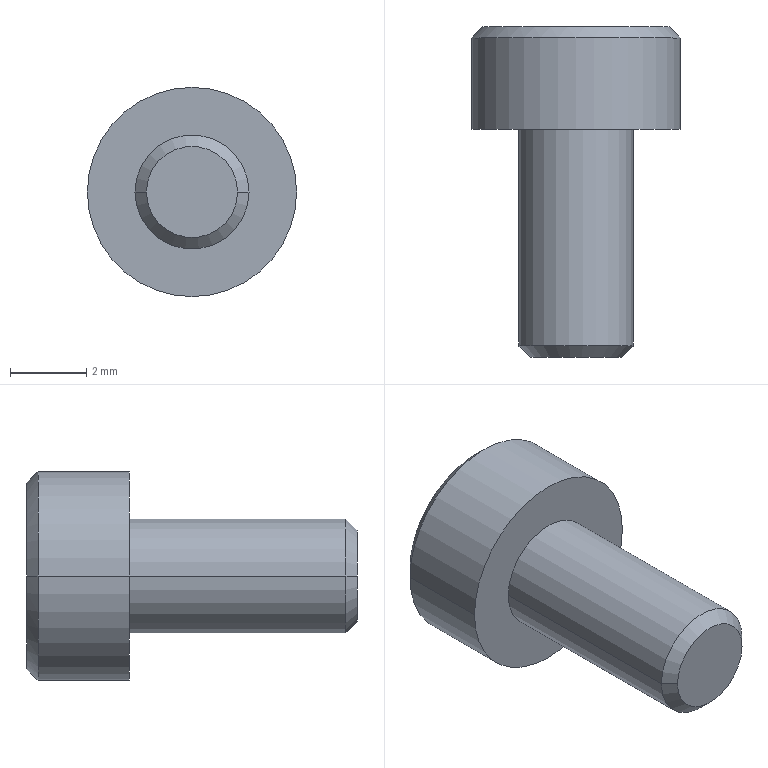Part | NX | 1 solid | 97 faces | box 5.5 x 8.7 x 5.5 mm | volume 96.053 mm3 | plane 87 | cone 6 | cylinder 4 | commonest cylinder face diameters 3 x2 5.5 x2